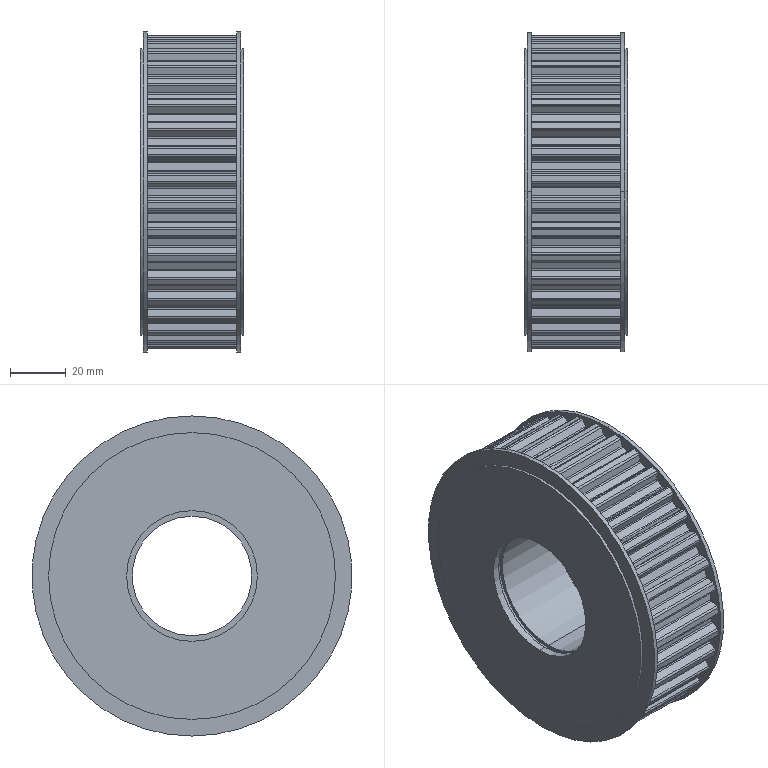Part | SolidWorks | features ICE 5, Fillet 2, CirPattern 1, Extrusion 1, MirrorPattern 1, RevCut 1 | 1 solid | 339 faces | box 37 x 115 x 115 mm | volume 284316 mm3 | cylinder 222 | plane 117 | commonest cylinder face diameters 1.6 x86 1.2 x84 112.74 x36 47 x4 103 x4 115 x4